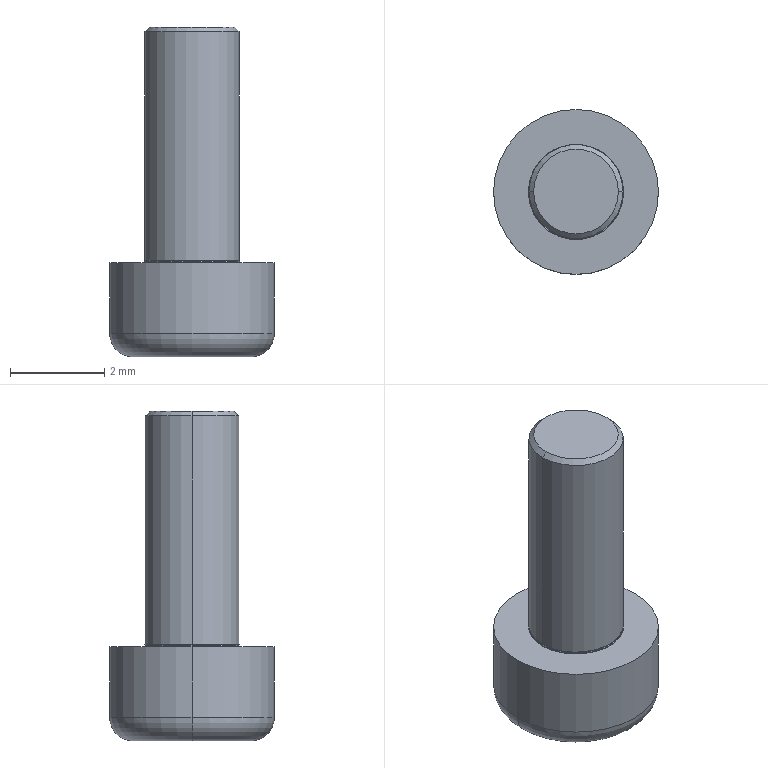Part | SolidWorks | features Attribute 1, Cut 1, Revolution 1 | 1 solid | 27 faces | box 3.5 x 3.5 x 7 mm | volume 32.905 mm3 | plane 11 | torus 6 | cylinder 6 | cone 4 | commonest cylinder face diameters 2 x4 3.5 x2
STEP:
#1=CARTESIAN_POINT('',(-1.013,0.,0.01));
#2=VERTEX_POINT('',#1);
#3=CARTESIAN_POINT('',(-0.9934,0.,0.03));
#4=VERTEX_POINT('',#3);
#5=CARTESIAN_POINT('',(-1.013,0.,0.03));
#6=DIRECTION('',(0.,-1.,0.));
#7=DIRECTION('',(0.,0.,-1.));
#8=AXIS2_PLACEMENT_3D('',#5,#6,#7);
#9=CIRCLE('',#8,0.02);
#10=EDGE_CURVE('',#2,#4,#9,.T.);
#11=ORIENTED_EDGE('',*,*,#10,.T.);
#12=CARTESIAN_POINT('',(0.9934,0.,0.03));
#13=VERTEX_POINT('',#12);
#14=CARTESIAN_POINT('',(0.,0.,0.03));
#15=DIRECTION('',(0.,0.,-1.));
#16=DIRECTION('',(-1.,0.,0.));
#17=AXIS2_PLACEMENT_3D('',#14,#15,#16);
#18=CIRCLE('',#17,0.9934);
#19=EDGE_CURVE('',#4,#13,#18,.T.);
#20=ORIENTED_EDGE('',*,*,#19,.T.);
#21=CARTESIAN_POINT('',(1.013,0.,0.01));
#22=VERTEX_POINT('',#21);
#23=CARTESIAN_POINT('',(1.013,0.,0.03));
#24=DIRECTION('',(0.,1.,0.));
#25=DIRECTION('',(-1.,0.,0.));
#26=AXIS2_PLACEMENT_3D('',#23,#24,#25);
#27=CIRCLE('',#26,0.02);
#28=EDGE_CURVE('',#22,#13,#27,.T.);
#29=ORIENTED_EDGE('',*,*,#28,.F.);
#30=CARTESIAN_POINT('',(0.,0.,0.01));
#31=DIRECTION('',(0.,0.,-1.));
#32=DIRECTION('',(-1.,0.,0.));
#33=AXIS2_PLACEMENT_3D('',#30,#31,#32);
#34=CIRCLE('',#33,1.013);
#35=EDGE_CURVE('',#2,#22,#34,.T.);
#36=ORIENTED_EDGE('',*,*,#35,.F.);
#37=EDGE_LOOP('',(#11,#20,#29,#36));
#38=FACE_OUTER_BOUND('',#37,.T.);
#39=CARTESIAN_POINT('',(0.,0.,0.03));
#40=DIRECTION('',(0.,0.,-1.));
#41=DIRECTION('',(-1.,0.,0.));
#42=AXIS2_PLACEMENT_3D('',#39,#40,#41);
#43=TOROIDAL_SURFACE('',#42,1.013,0.02);
#44=ADVANCED_FACE('',(#38),#43,.F.);
#45=ORIENTED_EDGE('',*,*,#28,.T.);
#46=CARTESIAN_POINT('',(0.,0.,0.03));
#47=DIRECTION('',(0.,0.,-1.));
#48=DIRECTION('',(-1.,0.,0.));
#49=AXIS2_PLACEMENT_3D('',#46,#47,#48);
#50=CIRCLE('',#49,0.9934);
#51=EDGE_CURVE('',#13,#4,#50,.T.);
#52=ORIENTED_EDGE('',*,*,#51,.T.);
#53=ORIENTED_EDGE('',*,*,#10,.F.);
#54=CARTESIAN_POINT('',(0.,0.,0.01));
#55=DIRECTION('',(0.,0.,-1.));
#56=DIRECTION('',(-1.,0.,0.));
#57=AXIS2_PLACEMENT_3D('',#54,#55,#56);
#58=CIRCLE('',#57,1.013);
#59=EDGE_CURVE('',#22,#2,#58,.T.);
#60=ORIENTED_EDGE('',*,*,#59,.F.);
#61=EDGE_LOOP('',(#45,#52,#53,#60));
#62=FACE_OUTER_BOUND('',#61,.T.);
#63=CARTESIAN_POINT('',(0.,0.,0.03));
#64=DIRECTION('',(0.,0.,-1.));
#65=DIRECTION('',(-1.,0.,0.));
#66=AXIS2_PLACEMENT_3D('',#63,#64,#65);
#67=TOROIDAL_SURFACE('',#66,1.013,0.02);
#68=ADVANCED_FACE('',(#62),#67,.F.);
#69=CARTESIAN_POINT('',(-0.9,0.,5.));
#70=VERTEX_POINT('',#69);
#71=CARTESIAN_POINT('',(0.9,0.,5.));
#72=VERTEX_POINT('',#71);
#73=CARTESIAN_POINT('',(0.,0.,5.));
#74=DIRECTION('',(0.,0.,-1.));
#75=DIRECTION('',(-1.,0.,0.));
#76=AXIS2_PLACEMENT_3D('',#73,#74,#75);
#77=CIRCLE('',#76,0.9);
#78=EDGE_CURVE('',#70,#72,#77,.T.);
#79=ORIENTED_EDGE('',*,*,#78,.T.);
#80=CARTESIAN_POINT('',(1.,0.,4.9));
#81=VERTEX_POINT('',#80);
#82=CARTESIAN_POINT('',(0.9,0.,5.));
#83=DIRECTION('',(0.7071,0.,-0.7071));
#84=VECTOR('',#83,1000.);
#85=LINE('',#82,#84);
#86=EDGE_CURVE('',#72,#81,#85,.T.);
#87=ORIENTED_EDGE('',*,*,#86,.T.);
#88=CARTESIAN_POINT('',(-1.,0.,4.9));
#89=VERTEX_POINT('',#88);
#90=CARTESIAN_POINT('',(0.,0.,4.9));
#91=DIRECTION('',(0.,0.,-1.));
#92=DIRECTION('',(-1.,0.,0.));
#93=AXIS2_PLACEMENT_3D('',#90,#91,#92);
#94=CIRCLE('',#93,1.);
#95=EDGE_CURVE('',#89,#81,#94,.T.);
#96=ORIENTED_EDGE('',*,*,#95,.F.);
#97=CARTESIAN_POINT('',(-0.9,0.,5.));
#98=DIRECTION('',(-0.7071,0.,-0.7071));
#99=VECTOR('',#98,1000.);
#100=LINE('',#97,#99);
#101=EDGE_CURVE('',#70,#89,#100,.T.);
#102=ORIENTED_EDGE('',*,*,#101,.F.);
#103=EDGE_LOOP('',(#79,#87,#96,#102));
#104=FACE_OUTER_BOUND('',#103,.T.);
#105=CARTESIAN_POINT('',(0.,0.,5.));
#106=DIRECTION('',(0.,0.,-1.));
#107=DIRECTION('',(-1.,0.,0.));
#108=AXIS2_PLACEMENT_3D('',#105,#106,#107);
#109=CONICAL_SURFACE('',#108,0.9,0.7854);
#110=ADVANCED_FACE('',(#104),#109,.T.);
#111=ORIENTED_EDGE('',*,*,#95,.T.);
#112=CARTESIAN_POINT('',(1.,0.,0.0464));
#113=VERTEX_POINT('',#112);
#114=CARTESIAN_POINT('',(1.,0.,-10.585));
#115=DIRECTION('',(0.,0.,-1.));
#116=VECTOR('',#115,1000.);
#117=LINE('',#114,#116);
#118=EDGE_CURVE('',#81,#113,#117,.T.);
#119=ORIENTED_EDGE('',*,*,#118,.T.);
#120=CARTESIAN_POINT('',(-1.,0.,0.0464));
#121=VERTEX_POINT('',#120);
#122=CARTESIAN_POINT('',(0.,0.,0.0464));
#123=DIRECTION('',(0.,0.,-1.));
#124=DIRECTION('',(-1.,0.,0.));
#125=AXIS2_PLACEMENT_3D('',#122,#123,#124);
#126=CIRCLE('',#125,1.);
#127=EDGE_CURVE('',#121,#113,#126,.T.);
#128=ORIENTED_EDGE('',*,*,#127,.F.);
#129=CARTESIAN_POINT('',(-1.,0.,-10.585));
#130=DIRECTION('',(0.,0.,-1.));
#131=VECTOR('',#130,1000.);
#132=LINE('',#129,#131);
#133=EDGE_CURVE('',#89,#121,#132,.T.);
#134=ORIENTED_EDGE('',*,*,#133,.F.);
#135=EDGE_LOOP('',(#111,#119,#128,#134));
#136=FACE_OUTER_BOUND('',#135,.T.);
#137=CARTESIAN_POINT('',(0.,0.,-10.585));
#138=DIRECTION('',(0.,0.,-1.));
#139=DIRECTION('',(-1.,0.,0.));
#140=AXIS2_PLACEMENT_3D('',#137,#138,#139);
#141=CYLINDRICAL_SURFACE('',#140,1.);
#142=ADVANCED_FACE('',(#136),#141,.T.);
#143=CARTESIAN_POINT('',(0.,0.,0.0464));
#144=DIRECTION('',(0.,0.,-1.));
#145=DIRECTION('',(-1.,0.,0.));
#146=AXIS2_PLACEMENT_3D('',#143,#144,#145);
#147=CIRCLE('',#146,1.);
#148=EDGE_CURVE('',#113,#121,#147,.T.);
#149=ORIENTED_EDGE('',*,*,#148,.T.);
#150=CARTESIAN_POINT('',(-1.007,0.,0.04879));
#151=VERTEX_POINT('',#150);
#152=CARTESIAN_POINT('',(-1.,0.,0.0464));
#153=DIRECTION('',(-0.9397,0.,0.342));
#154=VECTOR('',#153,1000.);
#155=LINE('',#152,#154);
#156=EDGE_CURVE('',#121,#151,#155,.T.);
#157=ORIENTED_EDGE('',*,*,#156,.T.);
#158=CARTESIAN_POINT('',(1.007,0.,0.04879));
#159=VERTEX_POINT('',#158);
#160=CARTESIAN_POINT('',(0.,0.,0.04879));
#161=DIRECTION('',(0.,0.,-1.));
#162=DIRECTION('',(-1.,0.,0.));
#163=AXIS2_PLACEMENT_3D('',#160,#161,#162);
#164=CIRCLE('',#163,1.007);
#165=EDGE_CURVE('',#159,#151,#164,.T.);
#166=ORIENTED_EDGE('',*,*,#165,.F.);
#167=CARTESIAN_POINT('',(1.,0.,0.0464));
#168=DIRECTION('',(0.9397,0.,0.342));
#169=VECTOR('',#168,1000.);
#170=LINE('',#167,#169);
#171=EDGE_CURVE('',#113,#159,#170,.T.);
#172=ORIENTED_EDGE('',*,*,#171,.F.);
#173=EDGE_LOOP('',(#149,#157,#166,#172));
#174=FACE_OUTER_BOUND('',#173,.T.);
#175=CARTESIAN_POINT('',(0.,0.,0.0464));
#176=DIRECTION('',(0.,0.,1.));
#177=DIRECTION('',(1.,0.,0.));
#178=AXIS2_PLACEMENT_3D('',#175,#176,#177);
#179=CONICAL_SURFACE('',#178,1.,1.222);
#180=ADVANCED_FACE('',(#174),#179,.F.);
#181=ORIENTED_EDGE('',*,*,#51,.F.);
#182=CARTESIAN_POINT('',(1.013,0.,0.03));
#183=DIRECTION('',(0.,1.,0.));
#184=DIRECTION('',(-1.,0.,0.));
#185=AXIS2_PLACEMENT_3D('',#182,#183,#184);
#186=CIRCLE('',#185,0.02);
#187=EDGE_CURVE('',#13,#159,#186,.T.);
#188=ORIENTED_EDGE('',*,*,#187,.T.);
#189=ORIENTED_EDGE('',*,*,#165,.T.);
#190=CARTESIAN_POINT('',(-1.013,0.,0.03));
#191=DIRECTION('',(0.,-1.,0.));
#192=DIRECTION('',(0.,0.,-1.));
#193=AXIS2_PLACEMENT_3D('',#190,#191,#192);
#194=CIRCLE('',#193,0.02);
#195=EDGE_CURVE('',#4,#151,#194,.T.);
#196=ORIENTED_EDGE('',*,*,#195,.F.);
#197=EDGE_LOOP('',(#181,#188,#189,#196));
#198=FACE_OUTER_BOUND('',#197,.T.);
#199=CARTESIAN_POINT('',(0.,0.,0.03));
#200=DIRECTION('',(0.,0.,-1.));
#201=DIRECTION('',(-1.,0.,0.));
#202=AXIS2_PLACEMENT_3D('',#199,#200,#201);
#203=TOROIDAL_SURFACE('',#202,1.013,0.02);
#204=ADVANCED_FACE('',(#198),#203,.F.);
#205=CARTESIAN_POINT('',(-1.,0.,0.01));
#206=VERTEX_POINT('',#205);
#207=CARTESIAN_POINT('',(1.,0.,0.01));
#208=VERTEX_POINT('',#207);
#209=CARTESIAN_POINT('',(0.,0.,0.01));
#210=DIRECTION('',(0.,0.,-1.));
#211=DIRECTION('',(-1.,0.,0.));
#212=AXIS2_PLACEMENT_3D('',#209,#210,#211);
#213=CIRCLE('',#212,1.);
#214=EDGE_CURVE('',#206,#208,#213,.T.);
#215=ORIENTED_EDGE('',*,*,#214,.T.);
#216=CARTESIAN_POINT('',(1.,0.,0.));
#217=VERTEX_POINT('',#216);
#218=CARTESIAN_POINT('',(1.,0.,-10.585));
#219=DIRECTION('',(0.,0.,-1.));
#220=VECTOR('',#219,1000.);
#221=LINE('',#218,#220);
#222=EDGE_CURVE('',#208,#217,#221,.T.);
#223=ORIENTED_EDGE('',*,*,#222,.T.);
#224=CARTESIAN_POINT('',(-1.,0.,0.));
#225=VERTEX_POINT('',#224);
#226=CARTESIAN_POINT('',(0.,0.,0.));
#227=DIRECTION('',(0.,0.,-1.));
#228=DIRECTION('',(-1.,0.,0.));
#229=AXIS2_PLACEMENT_3D('',#226,#227,#228);
#230=CIRCLE('',#229,1.);
#231=EDGE_CURVE('',#225,#217,#230,.T.);
#232=ORIENTED_EDGE('',*,*,#231,.F.);
#233=CARTESIAN_POINT('',(-1.,0.,-10.585));
#234=DIRECTION('',(0.,0.,-1.));
#235=VECTOR('',#234,1000.);
#236=LINE('',#233,#235);
#237=EDGE_CURVE('',#206,#225,#236,.T.);
#238=ORIENTED_EDGE('',*,*,#237,.F.);
#239=EDGE_LOOP('',(#215,#223,#232,#238));
#240=FACE_OUTER_BOUND('',#239,.T.);
#241=CARTESIAN_POINT('',(0.,0.,-10.585));
#242=DIRECTION('',(0.,0.,-1.));
#243=DIRECTION('',(-1.,0.,0.));
#244=AXIS2_PLACEMENT_3D('',#241,#242,#243);
#245=CYLINDRICAL_SURFACE('',#244,1.);
#246=ADVANCED_FACE('',(#240),#245,.T.);
#247=CARTESIAN_POINT('',(-1.75,0.,0.));
#248=VERTEX_POINT('',#247);
#249=CARTESIAN_POINT('',(1.75,0.,0.));
#250=VERTEX_POINT('',#249);
#251=CARTESIAN_POINT('',(0.,0.,0.));
#252=DIRECTION('',(0.,0.,-1.));
#253=DIRECTION('',(-1.,0.,0.));
#254=AXIS2_PLACEMENT_3D('',#251,#252,#253);
#255=CIRCLE('',#254,1.75);
#256=EDGE_CURVE('',#248,#250,#255,.T.);
#257=ORIENTED_EDGE('',*,*,#256,.T.);
#258=CARTESIAN_POINT('',(1.75,0.,-1.5));
#259=VERTEX_POINT('',#258);
#260=CARTESIAN_POINT('',(1.75,0.,-10.585));
#261=DIRECTION('',(0.,0.,-1.));
#262=VECTOR('',#261,1000.);
#263=LINE('',#260,#262);
#264=EDGE_CURVE('',#250,#259,#263,.T.);
#265=ORIENTED_EDGE('',*,*,#264,.T.);
#266=CARTESIAN_POINT('',(-1.75,0.,-1.5));
#267=VERTEX_POINT('',#266);
#268=CARTESIAN_POINT('',(0.,0.,-1.5));
#269=DIRECTION('',(0.,0.,-1.));
#270=DIRECTION('',(-1.,0.,0.));
#271=AXIS2_PLACEMENT_3D('',#268,#269,#270);
#272=CIRCLE('',#271,1.75);
#273=EDGE_CURVE('',#267,#259,#272,.T.);
#274=ORIENTED_EDGE('',*,*,#273,.F.);
#275=CARTESIAN_POINT('',(-1.75,0.,-10.585));
#276=DIRECTION('',(0.,0.,-1.));
#277=VECTOR('',#276,1000.);
#278=LINE('',#275,#277);
#279=EDGE_CURVE('',#248,#267,#278,.T.);
#280=ORIENTED_EDGE('',*,*,#279,.F.);
#281=EDGE_LOOP('',(#257,#265,#274,#280));
#282=FACE_OUTER_BOUND('',#281,.T.);
#283=CARTESIAN_POINT('',(0.,0.,-10.585));
#284=DIRECTION('',(0.,0.,-1.));
#285=DIRECTION('',(-1.,0.,0.));
#286=AXIS2_PLACEMENT_3D('',#283,#284,#285);
#287=CYLINDRICAL_SURFACE('',#286,1.75);
#288=ADVANCED_FACE('',(#282),#287,.T.);
#289=ORIENTED_EDGE('',*,*,#273,.T.);
#290=CARTESIAN_POINT('',(1.25,0.,-2.));
#291=VERTEX_POINT('',#290);
#292=CARTESIAN_POINT('',(1.25,0.,-1.5));
#293=DIRECTION('',(0.,1.,0.));
#294=DIRECTION('',(-1.,0.,0.));
#295=AXIS2_PLACEMENT_3D('',#292,#293,#294);
#296=CIRCLE('',#295,0.5);
#297=EDGE_CURVE('',#259,#291,#296,.T.);
#298=ORIENTED_EDGE('',*,*,#297,.T.);
#299=CARTESIAN_POINT('',(-1.25,0.,-2.));
#300=VERTEX_POINT('',#299);
#301=CARTESIAN_POINT('',(0.,0.,-2.));
#302=DIRECTION('',(0.,0.,-1.));
#303=DIRECTION('',(-1.,0.,0.));
#304=AXIS2_PLACEMENT_3D('',#301,#302,#303);
#305=CIRCLE('',#304,1.25);
#306=EDGE_CURVE('',#300,#291,#305,.T.);
#307=ORIENTED_EDGE('',*,*,#306,.F.);
#308=CARTESIAN_POINT('',(-1.25,0.,-1.5));
#309=DIRECTION('',(0.,-1.,0.));
#310=DIRECTION('',(0.,0.,-1.));
#311=AXIS2_PLACEMENT_3D('',#308,#309,#310);
#312=CIRCLE('',#311,0.5);
#313=EDGE_CURVE('',#267,#300,#312,.T.);
#314=ORIENTED_EDGE('',*,*,#313,.F.);
#315=EDGE_LOOP('',(#289,#298,#307,#314));
#316=FACE_OUTER_BOUND('',#315,.T.);
#317=CARTESIAN_POINT('',(0.,0.,-1.5));
#318=DIRECTION('',(0.,0.,-1.));
#319=DIRECTION('',(-1.,0.,0.));
#320=AXIS2_PLACEMENT_3D('',#317,#318,#319);
#321=TOROIDAL_SURFACE('',#320,1.25,0.5);
#322=ADVANCED_FACE('',(#316),#321,.T.);
#323=ORIENTED_EDGE('',*,*,#297,.F.);
#324=CARTESIAN_POINT('',(0.,0.,-1.5));
#325=DIRECTION('',(0.,0.,-1.));
#326=DIRECTION('',(-1.,0.,0.));
#327=AXIS2_PLACEMENT_3D('',#324,#325,#326);
#328=CIRCLE('',#327,1.75);
#329=EDGE_CURVE('',#259,#267,#328,.T.);
#330=ORIENTED_EDGE('',*,*,#329,.T.);
#331=ORIENTED_EDGE('',*,*,#313,.T.);
#332=CARTESIAN_POINT('',(0.,0.,-2.));
#333=DIRECTION('',(0.,0.,-1.));
#334=DIRECTION('',(-1.,0.,0.));
#335=AXIS2_PLACEMENT_3D('',#332,#333,#334);
#336=CIRCLE('',#335,1.25);
#337=EDGE_CURVE('',#291,#300,#336,.T.);
#338=ORIENTED_EDGE('',*,*,#337,.F.);
#339=EDGE_LOOP('',(#323,#330,#331,#338));
#340=FACE_OUTER_BOUND('',#339,.T.);
#341=CARTESIAN_POINT('',(0.,0.,-1.5));
#342=DIRECTION('',(0.,0.,-1.));
#343=DIRECTION('',(-1.,0.,0.));
#344=AXIS2_PLACEMENT_3D('',#341,#342,#343);
#345=TOROIDAL_SURFACE('',#344,1.25,0.5);
#346=ADVANCED_FACE('',(#340),#345,.T.);
#347=ORIENTED_EDGE('',*,*,#264,.F.);
#348=CARTESIAN_POINT('',(0.,0.,0.));
#349=DIRECTION('',(0.,0.,-1.));
#350=DIRECTION('',(-1.,0.,0.));
#351=AXIS2_PLACEMENT_3D('',#348,#349,#350);
#352=CIRCLE('',#351,1.75);
#353=EDGE_CURVE('',#250,#248,#352,.T.);
#354=ORIENTED_EDGE('',*,*,#353,.T.);
#355=ORIENTED_EDGE('',*,*,#279,.T.);
#356=ORIENTED_EDGE('',*,*,#329,.F.);
#357=EDGE_LOOP('',(#347,#354,#355,#356));
#358=FACE_OUTER_BOUND('',#357,.T.);
#359=CARTESIAN_POINT('',(0.,0.,-10.585));
#360=DIRECTION('',(0.,0.,-1.));
#361=DIRECTION('',(-1.,0.,0.));
#362=AXIS2_PLACEMENT_3D('',#359,#360,#361);
#363=CYLINDRICAL_SURFACE('',#362,1.75);
#364=ADVANCED_FACE('',(#358),#363,.T.);
#365=ORIENTED_EDGE('',*,*,#256,.F.);
#366=ORIENTED_EDGE('',*,*,#353,.F.);
#367=EDGE_LOOP('',(#365,#366));
#368=FACE_OUTER_BOUND('',#367,.T.);
#369=ORIENTED_EDGE('',*,*,#231,.T.);
#370=CARTESIAN_POINT('',(0.,0.,0.));
#371=DIRECTION('',(0.,0.,-1.));
#372=DIRECTION('',(-1.,0.,0.));
#373=AXIS2_PLACEMENT_3D('',#370,#371,#372);
#374=CIRCLE('',#373,1.);
#375=EDGE_CURVE('',#217,#225,#374,.T.);
#376=ORIENTED_EDGE('',*,*,#375,.T.);
#377=EDGE_LOOP('',(#369,#376));
#378=FACE_BOUND('',#377,.T.);
#379=CARTESIAN_POINT('',(-1.75,0.,0.));
#380=DIRECTION('',(0.,0.,-1.));
#381=DIRECTION('',(-1.,0.,0.));
#382=AXIS2_PLACEMENT_3D('',#379,#380,#381);
#383=PLANE('',#382);
#384=ADVANCED_FACE('',(#368,#378),#383,.F.);
#385=ORIENTED_EDGE('',*,*,#222,.F.);
#386=CARTESIAN_POINT('',(0.,0.,0.01));
#387=DIRECTION('',(0.,0.,-1.));
#388=DIRECTION('',(-1.,0.,0.));
#389=AXIS2_PLACEMENT_3D('',#386,#387,#388);
#390=CIRCLE('',#389,1.);
#391=EDGE_CURVE('',#208,#206,#390,.T.);
#392=ORIENTED_EDGE('',*,*,#391,.T.);
#393=ORIENTED_EDGE('',*,*,#237,.T.);
#394=ORIENTED_EDGE('',*,*,#375,.F.);
#395=EDGE_LOOP('',(#385,#392,#393,#394));
#396=FACE_OUTER_BOUND('',#395,.T.);
#397=CARTESIAN_POINT('',(0.,0.,-10.585));
#398=DIRECTION('',(0.,0.,-1.));
#399=DIRECTION('',(-1.,0.,0.));
#400=AXIS2_PLACEMENT_3D('',#397,#398,#399);
#401=CYLINDRICAL_SURFACE('',#400,1.);
#402=ADVANCED_FACE('',(#396),#401,.T.);
#403=ORIENTED_EDGE('',*,*,#214,.F.);
#404=ORIENTED_EDGE('',*,*,#391,.F.);
#405=EDGE_LOOP('',(#403,#404));
#406=FACE_BOUND('',#405,.T.);
#407=ORIENTED_EDGE('',*,*,#35,.T.);
#408=ORIENTED_EDGE('',*,*,#59,.T.);
#409=EDGE_LOOP('',(#407,#408));
#410=FACE_OUTER_BOUND('',#409,.T.);
#411=CARTESIAN_POINT('',(-1.,0.,0.01));
#412=DIRECTION('',(0.,0.,1.));
#413=DIRECTION('',(1.,0.,0.));
#414=AXIS2_PLACEMENT_3D('',#411,#412,#413);
#415=PLANE('',#414);
#416=ADVANCED_FACE('',(#406,#410),#415,.F.);
#417=ORIENTED_EDGE('',*,*,#19,.F.);
#418=ORIENTED_EDGE('',*,*,#195,.T.);
#419=CARTESIAN_POINT('',(0.,0.,0.04879));
#420=DIRECTION('',(0.,0.,-1.));
#421=DIRECTION('',(-1.,0.,0.));
#422=AXIS2_PLACEMENT_3D('',#419,#420,#421);
#423=CIRCLE('',#422,1.007);
#424=EDGE_CURVE('',#151,#159,#423,.T.);
#425=ORIENTED_EDGE('',*,*,#424,.T.);
#426=ORIENTED_EDGE('',*,*,#187,.F.);
#427=EDGE_LOOP('',(#417,#418,#425,#426));
#428=FACE_OUTER_BOUND('',#427,.T.);
#429=CARTESIAN_POINT('',(0.,0.,0.03));
#430=DIRECTION('',(0.,0.,-1.));
#431=DIRECTION('',(-1.,0.,0.));
#432=AXIS2_PLACEMENT_3D('',#429,#430,#431);
#433=TOROIDAL_SURFACE('',#432,1.013,0.02);
#434=ADVANCED_FACE('',(#428),#433,.F.);
#435=ORIENTED_EDGE('',*,*,#156,.F.);
#436=ORIENTED_EDGE('',*,*,#127,.T.);
#437=ORIENTED_EDGE('',*,*,#171,.T.);
#438=ORIENTED_EDGE('',*,*,#424,.F.);
#439=EDGE_LOOP('',(#435,#436,#437,#438));
#440=FACE_OUTER_BOUND('',#439,.T.);
#441=CARTESIAN_POINT('',(0.,0.,0.0464));
#442=DIRECTION('',(0.,0.,1.));
#443=DIRECTION('',(1.,0.,0.));
#444=AXIS2_PLACEMENT_3D('',#441,#442,#443);
#445=CONICAL_SURFACE('',#444,1.,1.222);
#446=ADVANCED_FACE('',(#440),#445,.F.);
#447=ORIENTED_EDGE('',*,*,#118,.F.);
#448=CARTESIAN_POINT('',(0.,0.,4.9));
#449=DIRECTION('',(0.,0.,-1.));
#450=DIRECTION('',(-1.,0.,0.));
#451=AXIS2_PLACEMENT_3D('',#448,#449,#450);
#452=CIRCLE('',#451,1.);
#453=EDGE_CURVE('',#81,#89,#452,.T.);
#454=ORIENTED_EDGE('',*,*,#453,.T.);
#455=ORIENTED_EDGE('',*,*,#133,.T.);
#456=ORIENTED_EDGE('',*,*,#148,.F.);
#457=EDGE_LOOP('',(#447,#454,#455,#456));
#458=FACE_OUTER_BOUND('',#457,.T.);
#459=CARTESIAN_POINT('',(0.,0.,-10.585));
#460=DIRECTION('',(0.,0.,-1.));
#461=DIRECTION('',(-1.,0.,0.));
#462=AXIS2_PLACEMENT_3D('',#459,#460,#461);
#463=CYLINDRICAL_SURFACE('',#462,1.);
#464=ADVANCED_FACE('',(#458),#463,.T.);
#465=ORIENTED_EDGE('',*,*,#86,.F.);
#466=CARTESIAN_POINT('',(0.,0.,5.));
#467=DIRECTION('',(0.,0.,-1.));
#468=DIRECTION('',(-1.,0.,0.));
#469=AXIS2_PLACEMENT_3D('',#466,#467,#468);
#470=CIRCLE('',#469,0.9);
#471=EDGE_CURVE('',#72,#70,#470,.T.);
#472=ORIENTED_EDGE('',*,*,#471,.T.);
#473=ORIENTED_EDGE('',*,*,#101,.T.);
#474=ORIENTED_EDGE('',*,*,#453,.F.);
#475=EDGE_LOOP('',(#465,#472,#473,#474));
#476=FACE_OUTER_BOUND('',#475,.T.);
#477=CARTESIAN_POINT('',(0.,0.,5.));
#478=DIRECTION('',(0.,0.,-1.));
#479=DIRECTION('',(-1.,0.,0.));
#480=AXIS2_PLACEMENT_3D('',#477,#478,#479);
#481=CONICAL_SURFACE('',#480,0.9,0.7854);
#482=ADVANCED_FACE('',(#476),#481,.T.);
#483=ORIENTED_EDGE('',*,*,#78,.F.);
#484=ORIENTED_EDGE('',*,*,#471,.F.);
#485=EDGE_LOOP('',(#483,#484));
#486=FACE_OUTER_BOUND('',#485,.T.);
#487=CARTESIAN_POINT('',(-0.9,0.,5.));
#488=DIRECTION('',(0.,0.,-1.));
#489=DIRECTION('',(-1.,0.,0.));
#490=AXIS2_PLACEMENT_3D('',#487,#488,#489);
#491=PLANE('',#490);
#492=ADVANCED_FACE('',(#486),#491,.F.);
#493=CARTESIAN_POINT('',(0.866,0.,-2.));
#494=VERTEX_POINT('',#493);
#495=CARTESIAN_POINT('',(0.433,-0.75,-2.));
#496=VERTEX_POINT('',#495);
#497=CARTESIAN_POINT('',(0.866,0.,-2.));
#498=DIRECTION('',(-0.5,-0.866,0.));
#499=VECTOR('',#498,1000.);
#500=LINE('',#497,#499);
#501=EDGE_CURVE('',#494,#496,#500,.T.);
#502=ORIENTED_EDGE('',*,*,#501,.F.);
#503=CARTESIAN_POINT('',(0.433,0.75,-2.));
#504=VERTEX_POINT('',#503);
#505=CARTESIAN_POINT('',(0.433,0.75,-2.));
#506=DIRECTION('',(0.5,-0.866,0.));
#507=VECTOR('',#506,1000.);
#508=LINE('',#505,#507);
#509=EDGE_CURVE('',#504,#494,#508,.T.);
#510=ORIENTED_EDGE('',*,*,#509,.F.);
#511=CARTESIAN_POINT('',(-0.433,0.75,-2.));
#512=VERTEX_POINT('',#511);
#513=CARTESIAN_POINT('',(-0.433,0.75,-2.));
#514=DIRECTION('',(1.,0.,0.));
#515=VECTOR('',#514,1000.);
#516=LINE('',#513,#515);
#517=EDGE_CURVE('',#512,#504,#516,.T.);
#518=ORIENTED_EDGE('',*,*,#517,.F.);
#519=CARTESIAN_POINT('',(-0.866,0.,-2.));
#520=VERTEX_POINT('',#519);
#521=CARTESIAN_POINT('',(-0.866,0.,-2.));
#522=DIRECTION('',(0.5,0.866,0.));
#523=VECTOR('',#522,1000.);
#524=LINE('',#521,#523);
#525=EDGE_CURVE('',#520,#512,#524,.T.);
#526=ORIENTED_EDGE('',*,*,#525,.F.);
#527=CARTESIAN_POINT('',(-0.433,-0.75,-2.));
#528=VERTEX_POINT('',#527);
#529=CARTESIAN_POINT('',(-0.433,-0.75,-2.));
#530=DIRECTION('',(-0.5,0.866,0.));
#531=VECTOR('',#530,1000.);
#532=LINE('',#529,#531);
#533=EDGE_CURVE('',#528,#520,#532,.T.);
#534=ORIENTED_EDGE('',*,*,#533,.F.);
#535=CARTESIAN_POINT('',(0.433,-0.75,-2.));
#536=DIRECTION('',(-1.,0.,0.));
#537=VECTOR('',#536,1000.);
#538=LINE('',#535,#537);
#539=EDGE_CURVE('',#496,#528,#538,.T.);
#540=ORIENTED_EDGE('',*,*,#539,.F.);
#541=EDGE_LOOP('',(#502,#510,#518,#526,#534,#540));
#542=FACE_BOUND('',#541,.T.);
#543=ORIENTED_EDGE('',*,*,#306,.T.);
#544=ORIENTED_EDGE('',*,*,#337,.T.);
#545=EDGE_LOOP('',(#543,#544));
#546=FACE_OUTER_BOUND('',#545,.T.);
#547=CARTESIAN_POINT('',(0.,0.,-2.));
#548=DIRECTION('',(0.,0.,1.));
#549=DIRECTION('',(1.,0.,0.));
#550=AXIS2_PLACEMENT_3D('',#547,#548,#549);
#551=PLANE('',#550);
#552=ADVANCED_FACE('',(#542,#546),#551,.F.);
#553=ORIENTED_EDGE('',*,*,#509,.T.);
#554=CARTESIAN_POINT('',(0.866,0.,-1.25));
#555=VERTEX_POINT('',#554);
#556=CARTESIAN_POINT('',(0.866,0.,-1.25));
#557=DIRECTION('',(0.,0.,-1.));
#558=VECTOR('',#557,1000.);
#559=LINE('',#556,#558);
#560=EDGE_CURVE('',#555,#494,#559,.T.);
#561=ORIENTED_EDGE('',*,*,#560,.F.);
#562=CARTESIAN_POINT('',(0.433,0.75,-1.25));
#563=VERTEX_POINT('',#562);
#564=CARTESIAN_POINT('',(0.433,0.75,-1.25));
#565=DIRECTION('',(0.5,-0.866,0.));
#566=VECTOR('',#565,1000.);
#567=LINE('',#564,#566);
#568=EDGE_CURVE('',#563,#555,#567,.T.);
#569=ORIENTED_EDGE('',*,*,#568,.F.);
#570=CARTESIAN_POINT('',(0.433,0.75,-1.25));
#571=DIRECTION('',(0.,0.,-1.));
#572=VECTOR('',#571,1000.);
#573=LINE('',#570,#572);
#574=EDGE_CURVE('',#563,#504,#573,.T.);
#575=ORIENTED_EDGE('',*,*,#574,.T.);
#576=EDGE_LOOP('',(#553,#561,#569,#575));
#577=FACE_OUTER_BOUND('',#576,.T.);
#578=CARTESIAN_POINT('',(0.433,0.75,-1.25));
#579=DIRECTION('',(0.866,0.5,0.));
#580=DIRECTION('',(-0.5,0.866,0.));
#581=AXIS2_PLACEMENT_3D('',#578,#579,#580);
#582=PLANE('',#581);
#583=ADVANCED_FACE('',(#577),#582,.F.);
#584=ORIENTED_EDGE('',*,*,#517,.T.);
#585=ORIENTED_EDGE('',*,*,#574,.F.);
#586=CARTESIAN_POINT('',(-0.433,0.75,-1.25));
#587=VERTEX_POINT('',#586);
#588=CARTESIAN_POINT('',(-0.433,0.75,-1.25));
#589=DIRECTION('',(1.,0.,0.));
#590=VECTOR('',#589,1000.);
#591=LINE('',#588,#590);
#592=EDGE_CURVE('',#587,#563,#591,.T.);
#593=ORIENTED_EDGE('',*,*,#592,.F.);
#594=CARTESIAN_POINT('',(-0.433,0.75,-1.25));
#595=DIRECTION('',(0.,0.,-1.));
#596=VECTOR('',#595,1000.);
#597=LINE('',#594,#596);
#598=EDGE_CURVE('',#587,#512,#597,.T.);
#599=ORIENTED_EDGE('',*,*,#598,.T.);
#600=EDGE_LOOP('',(#584,#585,#593,#599));
#601=FACE_OUTER_BOUND('',#600,.T.);
#602=CARTESIAN_POINT('',(-0.433,0.75,-1.25));
#603=DIRECTION('',(0.,1.,0.));
#604=DIRECTION('',(0.,0.,1.));
#605=AXIS2_PLACEMENT_3D('',#602,#603,#604);
#606=PLANE('',#605);
#607=ADVANCED_FACE('',(#601),#606,.F.);
#608=ORIENTED_EDGE('',*,*,#525,.T.);
#609=ORIENTED_EDGE('',*,*,#598,.F.);
#610=CARTESIAN_POINT('',(-0.866,0.,-1.25));
#611=VERTEX_POINT('',#610);
#612=CARTESIAN_POINT('',(-0.866,0.,-1.25));
#613=DIRECTION('',(0.5,0.866,0.));
#614=VECTOR('',#613,1000.);
#615=LINE('',#612,#614);
#616=EDGE_CURVE('',#611,#587,#615,.T.);
#617=ORIENTED_EDGE('',*,*,#616,.F.);
#618=CARTESIAN_POINT('',(-0.866,0.,-1.25));
#619=DIRECTION('',(0.,0.,-1.));
#620=VECTOR('',#619,1000.);
#621=LINE('',#618,#620);
#622=EDGE_CURVE('',#611,#520,#621,.T.);
#623=ORIENTED_EDGE('',*,*,#622,.T.);
#624=EDGE_LOOP('',(#608,#609,#617,#623));
#625=FACE_OUTER_BOUND('',#624,.T.);
#626=CARTESIAN_POINT('',(-0.866,0.,-1.25));
#627=DIRECTION('',(-0.866,0.5,0.));
#628=DIRECTION('',(-0.5,-0.866,0.));
#629=AXIS2_PLACEMENT_3D('',#626,#627,#628);
#630=PLANE('',#629);
#631=ADVANCED_FACE('',(#625),#630,.F.);
#632=ORIENTED_EDGE('',*,*,#533,.T.);
#633=ORIENTED_EDGE('',*,*,#622,.F.);
#634=CARTESIAN_POINT('',(-0.433,-0.75,-1.25));
#635=VERTEX_POINT('',#634);
#636=CARTESIAN_POINT('',(-0.433,-0.75,-1.25));
#637=DIRECTION('',(-0.5,0.866,0.));
#638=VECTOR('',#637,1000.);
#639=LINE('',#636,#638);
#640=EDGE_CURVE('',#635,#611,#639,.T.);
#641=ORIENTED_EDGE('',*,*,#640,.F.);
#642=CARTESIAN_POINT('',(-0.433,-0.75,-1.25));
#643=DIRECTION('',(0.,0.,-1.));
#644=VECTOR('',#643,1000.);
#645=LINE('',#642,#644);
#646=EDGE_CURVE('',#635,#528,#645,.T.);
#647=ORIENTED_EDGE('',*,*,#646,.T.);
#648=EDGE_LOOP('',(#632,#633,#641,#647));
#649=FACE_OUTER_BOUND('',#648,.T.);
#650=CARTESIAN_POINT('',(-0.433,-0.75,-1.25));
#651=DIRECTION('',(-0.866,-0.5,0.));
#652=DIRECTION('',(0.5,-0.866,0.));
#653=AXIS2_PLACEMENT_3D('',#650,#651,#652);
#654=PLANE('',#653);
#655=ADVANCED_FACE('',(#649),#654,.F.);
#656=ORIENTED_EDGE('',*,*,#539,.T.);
#657=ORIENTED_EDGE('',*,*,#646,.F.);
#658=CARTESIAN_POINT('',(0.433,-0.75,-1.25));
#659=VERTEX_POINT('',#658);
#660=CARTESIAN_POINT('',(0.433,-0.75,-1.25));
#661=DIRECTION('',(-1.,0.,0.));
#662=VECTOR('',#661,1000.);
#663=LINE('',#660,#662);
#664=EDGE_CURVE('',#659,#635,#663,.T.);
#665=ORIENTED_EDGE('',*,*,#664,.F.);
#666=CARTESIAN_POINT('',(0.433,-0.75,-1.25));
#667=DIRECTION('',(0.,0.,-1.));
#668=VECTOR('',#667,1000.);
#669=LINE('',#666,#668);
#670=EDGE_CURVE('',#659,#496,#669,.T.);
#671=ORIENTED_EDGE('',*,*,#670,.T.);
#672=EDGE_LOOP('',(#656,#657,#665,#671));
#673=FACE_OUTER_BOUND('',#672,.T.);
#674=CARTESIAN_POINT('',(0.433,-0.75,-1.25));
#675=DIRECTION('',(0.,-1.,0.));
#676=DIRECTION('',(0.,0.,-1.));
#677=AXIS2_PLACEMENT_3D('',#674,#675,#676);
#678=PLANE('',#677);
#679=ADVANCED_FACE('',(#673),#678,.F.);
#680=ORIENTED_EDGE('',*,*,#501,.T.);
#681=ORIENTED_EDGE('',*,*,#670,.F.);
#682=CARTESIAN_POINT('',(0.866,0.,-1.25));
#683=DIRECTION('',(-0.5,-0.866,0.));
#684=VECTOR('',#683,1000.);
#685=LINE('',#682,#684);
#686=EDGE_CURVE('',#555,#659,#685,.T.);
#687=ORIENTED_EDGE('',*,*,#686,.F.);
#688=ORIENTED_EDGE('',*,*,#560,.T.);
#689=EDGE_LOOP('',(#680,#681,#687,#688));
#690=FACE_OUTER_BOUND('',#689,.T.);
#691=CARTESIAN_POINT('',(0.866,0.,-1.25));
#692=DIRECTION('',(0.866,-0.5,0.));
#693=DIRECTION('',(0.5,0.866,0.));
#694=AXIS2_PLACEMENT_3D('',#691,#692,#693);
#695=PLANE('',#694);
#696=ADVANCED_FACE('',(#690),#695,.F.);
#697=ORIENTED_EDGE('',*,*,#568,.T.);
#698=ORIENTED_EDGE('',*,*,#686,.T.);
#699=ORIENTED_EDGE('',*,*,#664,.T.);
#700=ORIENTED_EDGE('',*,*,#640,.T.);
#701=ORIENTED_EDGE('',*,*,#616,.T.);
#702=ORIENTED_EDGE('',*,*,#592,.T.);
#703=EDGE_LOOP('',(#697,#698,#699,#700,#701,#702));
#704=FACE_OUTER_BOUND('',#703,.T.);
#705=CARTESIAN_POINT('',(1.299,-0.75,-1.25));
#706=DIRECTION('',(0.,0.,-1.));
#707=DIRECTION('',(-1.,0.,0.));
#708=AXIS2_PLACEMENT_3D('',#705,#706,#707);
#709=PLANE('',#708);
#710=ADVANCED_FACE('',(#704),#709,.T.);
#711=CLOSED_SHELL('',(#44,#68,#110,#142,#180,#204,#246,#288,#322,#346,#364,#384,#402,#416,#434,#446,#464,#482,#492,#552,#583,#607,#631,#655,#679,#696,#710));
#712=MANIFOLD_SOLID_BREP('',#711);
#713=CARTESIAN_POINT('',(0.,0.,0.));
#714=DIRECTION('',(0.,0.,1.));
#715=DIRECTION('',(1.,0.,0.));
#716=AXIS2_PLACEMENT_3D('',#713,#714,#715);
#717=(LENGTH_UNIT()NAMED_UNIT(*)SI_UNIT(.MILLI.,.METRE.));
#718=UNCERTAINTY_MEASURE_WITH_UNIT(LENGTH_MEASURE(0.00001),#717,'','');
#719=(NAMED_UNIT(*)PLANE_ANGLE_UNIT()SI_UNIT($,.RADIAN.));
#720=(NAMED_UNIT(*)SI_UNIT($,.STERADIAN.)SOLID_ANGLE_UNIT());
#721=(GEOMETRIC_REPRESENTATION_CONTEXT(3)GLOBAL_UNCERTAINTY_ASSIGNED_CONTEXT((#718))GLOBAL_UNIT_ASSIGNED_CONTEXT((#717,#719,#720))REPRESENTATION_CONTEXT('',''));
#722=ADVANCED_BREP_SHAPE_REPRESENTATION('',(#712,#716),#721);